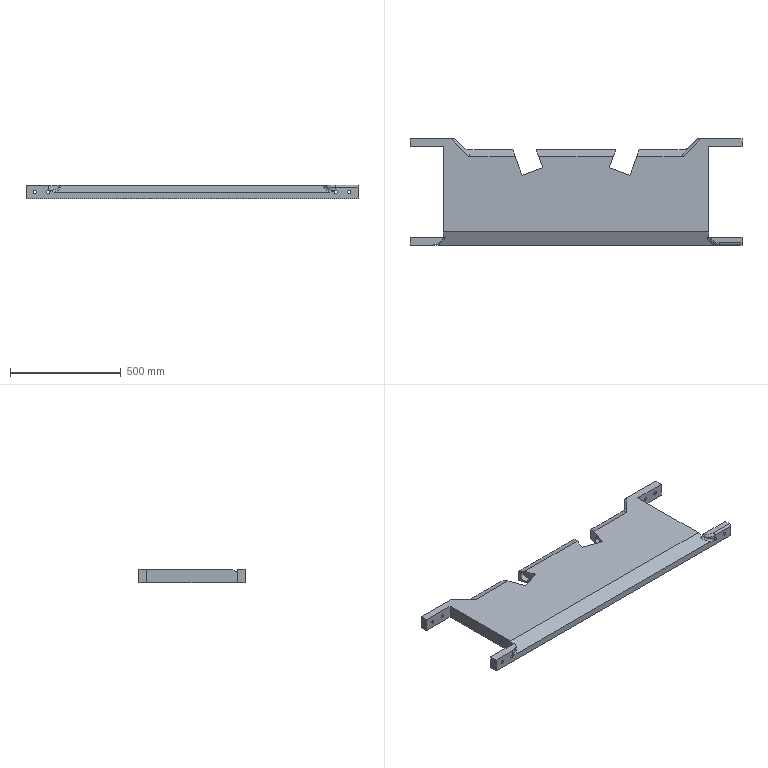Part | SolidWorks | features Fillet 5, ICE 4, Chamfer 2, Cut 1, Extrusion 1, MirrorPattern 1 | 1 solid | 71 faces | box 1500 x 480 x 60 mm | volume 30002400 mm3 | plane 36 | cylinder 31 | spline 3 | torus 1 | commonest cylinder face diameters 15 x16 45 x8 100 x4 20 x3